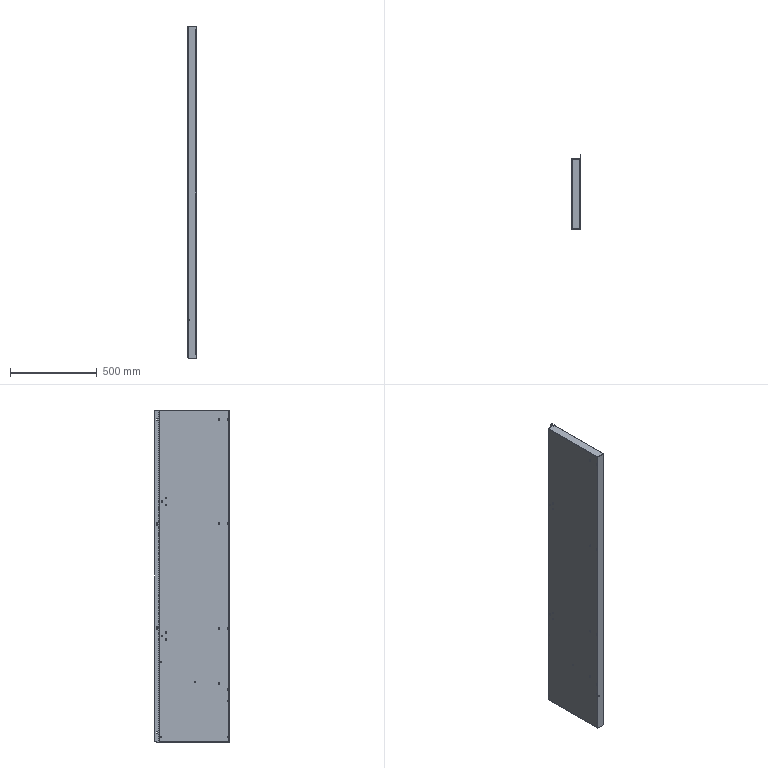Part | SolidWorks | 1 solid | 180 faces | box 50 x 430 x 1914 mm | volume 1681959 mm3 | plane 100 | cylinder 80 | commonest cylinder face diameters 6 x16 6.4 x12 7 x12 8.5 x12 2 x9 5 x9